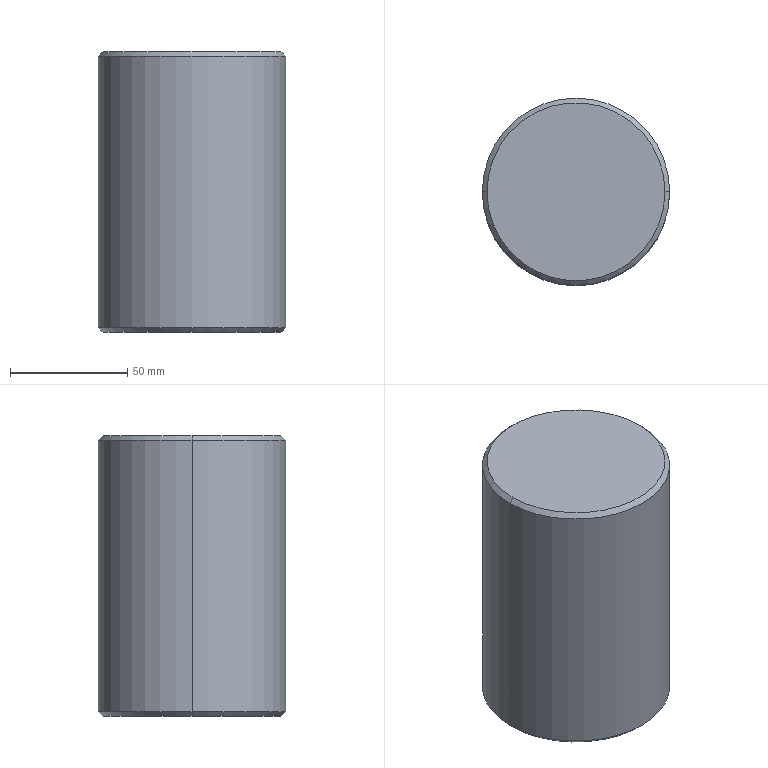Part | STEP file | 4-20.sldasm-Part-325 | 1 solid | 8 faces | box 80 x 80 x 120 mm | volume 602197 mm3 | cone 4 | cylinder 2 | plane 2 | commonest cylinder face diameters 80 x2
STEP:
#1=CARTESIAN_POINT('',(33.,-150.,-20.));
#2=VERTEX_POINT('',#1);
#3=CARTESIAN_POINT('',(-43.,-150.,-20.));
#4=VERTEX_POINT('',#3);
#5=CARTESIAN_POINT('',(-5.,-150.,-20.));
#6=DIRECTION('',(0.,0.,1.));
#7=DIRECTION('',(1.,0.,0.));
#8=AXIS2_PLACEMENT_3D('',#5,#6,#7);
#9=CIRCLE('',#8,38.);
#10=EDGE_CURVE('',#2,#4,#9,.T.);
#11=ORIENTED_EDGE('',*,*,#10,.F.);
#12=CARTESIAN_POINT('',(35.,-150.,-22.));
#13=VERTEX_POINT('',#12);
#14=CARTESIAN_POINT('',(35.,-150.,-22.));
#15=DIRECTION('',(0.7071,0.,-0.7071));
#16=VECTOR('',#15,1000.);
#17=LINE('',#14,#16);
#18=EDGE_CURVE('',#2,#13,#17,.T.);
#19=ORIENTED_EDGE('',*,*,#18,.T.);
#20=CARTESIAN_POINT('',(-45.,-150.,-22.));
#21=VERTEX_POINT('',#20);
#22=CARTESIAN_POINT('',(-5.,-150.,-22.));
#23=DIRECTION('',(0.,0.,-1.));
#24=DIRECTION('',(1.,0.,0.));
#25=AXIS2_PLACEMENT_3D('',#22,#23,#24);
#26=CIRCLE('',#25,40.);
#27=EDGE_CURVE('',#21,#13,#26,.T.);
#28=ORIENTED_EDGE('',*,*,#27,.F.);
#29=CARTESIAN_POINT('',(-45.,-150.,-22.));
#30=DIRECTION('',(-0.7071,0.,-0.7071));
#31=VECTOR('',#30,1000.);
#32=LINE('',#29,#31);
#33=EDGE_CURVE('',#4,#21,#32,.T.);
#34=ORIENTED_EDGE('',*,*,#33,.F.);
#35=EDGE_LOOP('',(#11,#19,#28,#34));
#36=FACE_OUTER_BOUND('',#35,.T.);
#37=CARTESIAN_POINT('',(-5.,-150.,-22.));
#38=DIRECTION('',(0.,0.,-1.));
#39=DIRECTION('',(-1.,0.,0.));
#40=AXIS2_PLACEMENT_3D('',#37,#38,#39);
#41=CONICAL_SURFACE('',#40,40.,0.7854);
#42=ADVANCED_FACE('',(#36),#41,.T.);
#43=CARTESIAN_POINT('',(-43.,-150.,-140.));
#44=VERTEX_POINT('',#43);
#45=CARTESIAN_POINT('',(33.,-150.,-140.));
#46=VERTEX_POINT('',#45);
#47=CARTESIAN_POINT('',(-5.,-150.,-140.));
#48=DIRECTION('',(0.,0.,-1.));
#49=DIRECTION('',(1.,0.,0.));
#50=AXIS2_PLACEMENT_3D('',#47,#48,#49);
#51=CIRCLE('',#50,38.);
#52=EDGE_CURVE('',#44,#46,#51,.T.);
#53=ORIENTED_EDGE('',*,*,#52,.F.);
#54=CARTESIAN_POINT('',(-45.,-150.,-138.));
#55=VERTEX_POINT('',#54);
#56=CARTESIAN_POINT('',(-45.,-150.,-138.));
#57=DIRECTION('',(-0.7071,0.,0.7071));
#58=VECTOR('',#57,1000.);
#59=LINE('',#56,#58);
#60=EDGE_CURVE('',#44,#55,#59,.T.);
#61=ORIENTED_EDGE('',*,*,#60,.T.);
#62=CARTESIAN_POINT('',(35.,-150.,-138.));
#63=VERTEX_POINT('',#62);
#64=CARTESIAN_POINT('',(-5.,-150.,-138.));
#65=DIRECTION('',(0.,0.,1.));
#66=DIRECTION('',(1.,0.,0.));
#67=AXIS2_PLACEMENT_3D('',#64,#65,#66);
#68=CIRCLE('',#67,40.);
#69=EDGE_CURVE('',#63,#55,#68,.T.);
#70=ORIENTED_EDGE('',*,*,#69,.F.);
#71=CARTESIAN_POINT('',(35.,-150.,-138.));
#72=DIRECTION('',(0.7071,0.,0.7071));
#73=VECTOR('',#72,1000.);
#74=LINE('',#71,#73);
#75=EDGE_CURVE('',#46,#63,#74,.T.);
#76=ORIENTED_EDGE('',*,*,#75,.F.);
#77=EDGE_LOOP('',(#53,#61,#70,#76));
#78=FACE_OUTER_BOUND('',#77,.T.);
#79=CARTESIAN_POINT('',(-5.,-150.,-138.));
#80=DIRECTION('',(0.,0.,1.));
#81=DIRECTION('',(1.,0.,0.));
#82=AXIS2_PLACEMENT_3D('',#79,#80,#81);
#83=CONICAL_SURFACE('',#82,40.,0.7854);
#84=ADVANCED_FACE('',(#78),#83,.T.);
#85=ORIENTED_EDGE('',*,*,#69,.T.);
#86=CARTESIAN_POINT('',(-45.,-150.,-679.868));
#87=DIRECTION('',(0.,0.,1.));
#88=VECTOR('',#87,1000.);
#89=LINE('',#86,#88);
#90=EDGE_CURVE('',#55,#21,#89,.T.);
#91=ORIENTED_EDGE('',*,*,#90,.T.);
#92=ORIENTED_EDGE('',*,*,#27,.T.);
#93=CARTESIAN_POINT('',(35.,-150.,-679.868));
#94=DIRECTION('',(0.,0.,1.));
#95=VECTOR('',#94,1000.);
#96=LINE('',#93,#95);
#97=EDGE_CURVE('',#63,#13,#96,.T.);
#98=ORIENTED_EDGE('',*,*,#97,.F.);
#99=EDGE_LOOP('',(#85,#91,#92,#98));
#100=FACE_OUTER_BOUND('',#99,.T.);
#101=CARTESIAN_POINT('',(-5.,-150.,-679.868));
#102=DIRECTION('',(0.,0.,1.));
#103=DIRECTION('',(1.,0.,0.));
#104=AXIS2_PLACEMENT_3D('',#101,#102,#103);
#105=CYLINDRICAL_SURFACE('',#104,40.);
#106=ADVANCED_FACE('',(#100),#105,.T.);
#107=CARTESIAN_POINT('',(-5.,-150.,-140.));
#108=DIRECTION('',(0.,0.,-1.));
#109=DIRECTION('',(1.,0.,0.));
#110=AXIS2_PLACEMENT_3D('',#107,#108,#109);
#111=CIRCLE('',#110,38.);
#112=EDGE_CURVE('',#46,#44,#111,.T.);
#113=ORIENTED_EDGE('',*,*,#112,.T.);
#114=ORIENTED_EDGE('',*,*,#52,.T.);
#115=EDGE_LOOP('',(#113,#114));
#116=FACE_OUTER_BOUND('',#115,.T.);
#117=CARTESIAN_POINT('',(-421.067,818.4,-140.));
#118=DIRECTION('',(0.,0.,1.));
#119=DIRECTION('',(0.,1.,0.));
#120=AXIS2_PLACEMENT_3D('',#117,#118,#119);
#121=PLANE('',#120);
#122=ADVANCED_FACE('',(#116),#121,.F.);
#123=ORIENTED_EDGE('',*,*,#90,.F.);
#124=CARTESIAN_POINT('',(-5.,-150.,-138.));
#125=DIRECTION('',(0.,0.,1.));
#126=DIRECTION('',(1.,0.,0.));
#127=AXIS2_PLACEMENT_3D('',#124,#125,#126);
#128=CIRCLE('',#127,40.);
#129=EDGE_CURVE('',#55,#63,#128,.T.);
#130=ORIENTED_EDGE('',*,*,#129,.T.);
#131=ORIENTED_EDGE('',*,*,#97,.T.);
#132=CARTESIAN_POINT('',(-5.,-150.,-22.));
#133=DIRECTION('',(0.,0.,-1.));
#134=DIRECTION('',(1.,0.,0.));
#135=AXIS2_PLACEMENT_3D('',#132,#133,#134);
#136=CIRCLE('',#135,40.);
#137=EDGE_CURVE('',#13,#21,#136,.T.);
#138=ORIENTED_EDGE('',*,*,#137,.T.);
#139=EDGE_LOOP('',(#123,#130,#131,#138));
#140=FACE_OUTER_BOUND('',#139,.T.);
#141=CARTESIAN_POINT('',(-5.,-150.,-679.868));
#142=DIRECTION('',(0.,0.,1.));
#143=DIRECTION('',(1.,0.,0.));
#144=AXIS2_PLACEMENT_3D('',#141,#142,#143);
#145=CYLINDRICAL_SURFACE('',#144,40.);
#146=ADVANCED_FACE('',(#140),#145,.T.);
#147=CARTESIAN_POINT('',(-5.,-150.,-20.));
#148=DIRECTION('',(0.,0.,1.));
#149=DIRECTION('',(1.,0.,0.));
#150=AXIS2_PLACEMENT_3D('',#147,#148,#149);
#151=CIRCLE('',#150,38.);
#152=EDGE_CURVE('',#4,#2,#151,.T.);
#153=ORIENTED_EDGE('',*,*,#152,.T.);
#154=ORIENTED_EDGE('',*,*,#10,.T.);
#155=EDGE_LOOP('',(#153,#154));
#156=FACE_OUTER_BOUND('',#155,.T.);
#157=CARTESIAN_POINT('',(-5.,-150.,-20.));
#158=DIRECTION('',(0.,0.,1.));
#159=DIRECTION('',(1.,0.,0.));
#160=AXIS2_PLACEMENT_3D('',#157,#158,#159);
#161=PLANE('',#160);
#162=ADVANCED_FACE('',(#156),#161,.T.);
#163=ORIENTED_EDGE('',*,*,#60,.F.);
#164=ORIENTED_EDGE('',*,*,#112,.F.);
#165=ORIENTED_EDGE('',*,*,#75,.T.);
#166=ORIENTED_EDGE('',*,*,#129,.F.);
#167=EDGE_LOOP('',(#163,#164,#165,#166));
#168=FACE_OUTER_BOUND('',#167,.T.);
#169=CARTESIAN_POINT('',(-5.,-150.,-138.));
#170=DIRECTION('',(0.,0.,1.));
#171=DIRECTION('',(1.,0.,0.));
#172=AXIS2_PLACEMENT_3D('',#169,#170,#171);
#173=CONICAL_SURFACE('',#172,40.,0.7854);
#174=ADVANCED_FACE('',(#168),#173,.T.);
#175=ORIENTED_EDGE('',*,*,#18,.F.);
#176=ORIENTED_EDGE('',*,*,#152,.F.);
#177=ORIENTED_EDGE('',*,*,#33,.T.);
#178=ORIENTED_EDGE('',*,*,#137,.F.);
#179=EDGE_LOOP('',(#175,#176,#177,#178));
#180=FACE_OUTER_BOUND('',#179,.T.);
#181=CARTESIAN_POINT('',(-5.,-150.,-22.));
#182=DIRECTION('',(0.,0.,-1.));
#183=DIRECTION('',(-1.,0.,0.));
#184=AXIS2_PLACEMENT_3D('',#181,#182,#183);
#185=CONICAL_SURFACE('',#184,40.,0.7854);
#186=ADVANCED_FACE('',(#180),#185,.T.);
#187=CLOSED_SHELL('',(#42,#84,#106,#122,#146,#162,#174,#186));
#188=MANIFOLD_SOLID_BREP('',#187);
#189=CARTESIAN_POINT('',(0.,0.,0.));
#190=DIRECTION('',(0.,0.,1.));
#191=DIRECTION('',(1.,0.,0.));
#192=AXIS2_PLACEMENT_3D('',#189,#190,#191);
#193=(LENGTH_UNIT()NAMED_UNIT(*)SI_UNIT(.MILLI.,.METRE.));
#194=UNCERTAINTY_MEASURE_WITH_UNIT(LENGTH_MEASURE(0.00001),#193,'','');
#195=(NAMED_UNIT(*)PLANE_ANGLE_UNIT()SI_UNIT($,.RADIAN.));
#196=(NAMED_UNIT(*)SI_UNIT($,.STERADIAN.)SOLID_ANGLE_UNIT());
#197=(GEOMETRIC_REPRESENTATION_CONTEXT(3)GLOBAL_UNCERTAINTY_ASSIGNED_CONTEXT((#194))GLOBAL_UNIT_ASSIGNED_CONTEXT((#193,#195,#196))REPRESENTATION_CONTEXT('',''));
#198=ADVANCED_BREP_SHAPE_REPRESENTATION('',(#188,#192),#197);